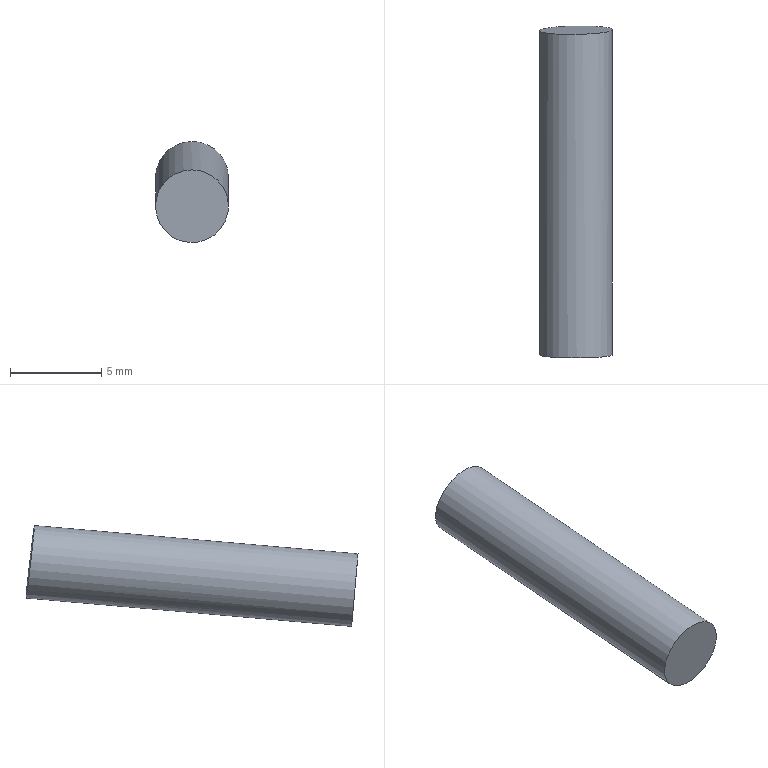Part | NX | features solid 2 | 1 solid | 3 faces | box 4 x 18.195 x 5.536 mm | volume 224.361 mm3 | plane 2 | cylinder 1 | commonest cylinder face diameters 4 x1
STEP:
#1=CARTESIAN_POINT('',(-174.498,40.515,-44.863));
#2=VERTEX_POINT('',#1);
#3=CARTESIAN_POINT('',(-172.498,40.515,-44.863));
#4=DIRECTION('',(0.,0.9962,0.08716));
#5=DIRECTION('',(-1.,0.,0.));
#6=AXIS2_PLACEMENT_3D('',#3,#4,#5);
#7=CIRCLE('',#6,2.);
#8=EDGE_CURVE('',#2,#2,#7,.T.);
#9=ORIENTED_EDGE('',*,*,#8,.F.);
#10=EDGE_LOOP('',(#9));
#11=FACE_BOUND('',#10,.T.);
#12=CARTESIAN_POINT('',(-172.498,40.515,-44.863));
#13=DIRECTION('',(0.,-0.9962,-0.08716));
#14=DIRECTION('',(1.,0.,0.));
#15=AXIS2_PLACEMENT_3D('',#12,#13,#14);
#16=PLANE('',#15);
#17=ADVANCED_FACE('',(#11),#16,.T.);
#18=CARTESIAN_POINT('',(-173.421,58.081,-41.545));
#19=VERTEX_POINT('',#18);
#20=CARTESIAN_POINT('',(-172.498,58.301,-43.307));
#21=DIRECTION('',(-0.01517,0.9931,0.1162));
#22=DIRECTION('',(-0.4611,-0.11,0.8805));
#23=AXIS2_PLACEMENT_3D('',#20,#21,#22);
#24=ELLIPSE('',#23,2.001,2.);
#25=EDGE_CURVE('',#19,#19,#24,.F.);
#26=ORIENTED_EDGE('',*,*,#25,.F.);
#27=EDGE_LOOP('',(#26));
#28=FACE_BOUND('',#27,.T.);
#29=CARTESIAN_POINT('',(-173.425,42.623,90.607));
#30=DIRECTION('',(-0.01517,0.9931,0.1162));
#31=DIRECTION('',(0.05188,0.1168,-0.9918));
#32=AXIS2_PLACEMENT_3D('',#29,#30,#31);
#33=PLANE('',#32);
#34=ADVANCED_FACE('',(#28),#33,.T.);
#35=ORIENTED_EDGE('',*,*,#8,.T.);
#36=EDGE_LOOP('',(#35));
#37=FACE_BOUND('',#36,.T.);
#38=ORIENTED_EDGE('',*,*,#25,.T.);
#39=EDGE_LOOP('',(#38));
#40=FACE_BOUND('',#39,.T.);
#41=CARTESIAN_POINT('',(-172.498,60.439,-43.12));
#42=DIRECTION('',(0.,-0.9962,-0.08716));
#43=DIRECTION('',(1.,0.,0.));
#44=AXIS2_PLACEMENT_3D('',#41,#42,#43);
#45=CYLINDRICAL_SURFACE('',#44,2.);
#46=ADVANCED_FACE('',(#37,#40),#45,.T.);
#47=CLOSED_SHELL('',(#17,#34,#46));
#48=MANIFOLD_SOLID_BREP('',#47);
#49=(LENGTH_UNIT()NAMED_UNIT(*)SI_UNIT(.MILLI.,.METRE.));
#50=UNCERTAINTY_MEASURE_WITH_UNIT(LENGTH_MEASURE(0.00001),#49,'','');
#51=(NAMED_UNIT(*)PLANE_ANGLE_UNIT()SI_UNIT($,.RADIAN.));
#52=(NAMED_UNIT(*)SI_UNIT($,.STERADIAN.)SOLID_ANGLE_UNIT());
#53=(GEOMETRIC_REPRESENTATION_CONTEXT(3)GLOBAL_UNCERTAINTY_ASSIGNED_CONTEXT((#50))GLOBAL_UNIT_ASSIGNED_CONTEXT((#49,#51,#52))REPRESENTATION_CONTEXT('',''));
#54=ADVANCED_BREP_SHAPE_REPRESENTATION('',(#48),#53);